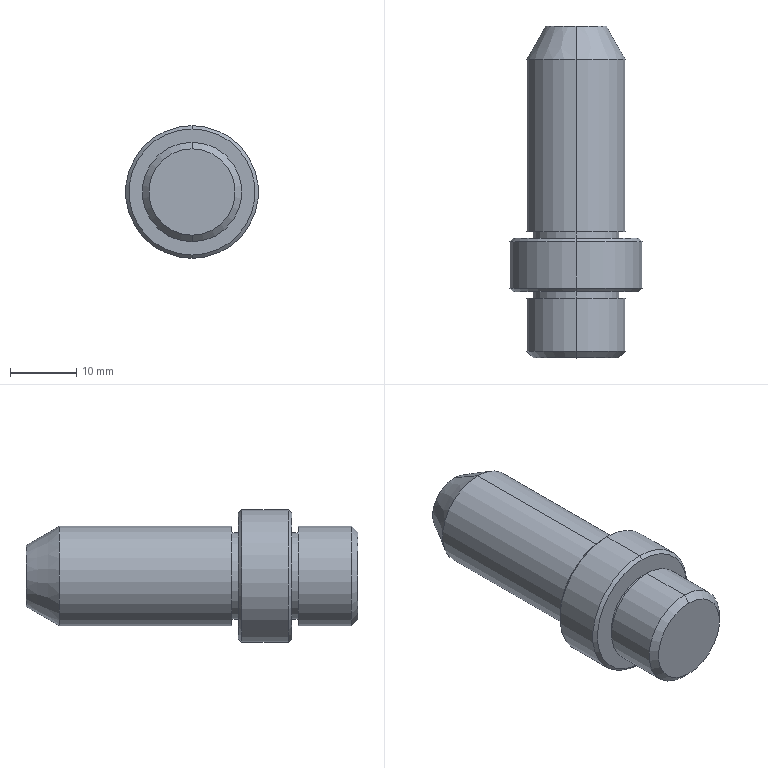Part | STEP file | Locating Pin | 1 solid | 24 faces | box 20 x 50 x 20 mm | volume 9513 mm3 | cylinder 10 | cone 8 | plane 6 | commonest cylinder face diameters 13 x4 15 x4 20 x2
STEP:
#1=CARTESIAN_POINT('',(0.,0.,0.));
#2=DIRECTION('',(0.,0.,1.));
#3=DIRECTION('',(1.,0.,0.));
#4=AXIS2_PLACEMENT_3D('',#1,#2,#3);
#5=CARTESIAN_POINT('',(18051.815,6151.815,9.5));
#6=VERTEX_POINT('',#5);
#7=CARTESIAN_POINT('',(18051.815,6151.815,-9.5));
#8=VERTEX_POINT('',#7);
#9=CARTESIAN_POINT('',(18051.815,6151.815,0.));
#10=DIRECTION('',(0.,1.,0.));
#11=DIRECTION('',(0.,0.,-1.));
#12=AXIS2_PLACEMENT_3D('',#9,#10,#11);
#13=CIRCLE('',#12,9.5);
#14=CARTESIAN_POINT('',(18051.815,6151.315,0.));
#15=DIRECTION('',(0.,-1.,0.));
#16=DIRECTION('',(0.,0.,-1.));
#17=AXIS2_PLACEMENT_3D('',#14,#15,#16);
#18=CONICAL_SURFACE('',#17,10.,0.7854);
#19=CARTESIAN_POINT('',(6.283,-0.5));
#20=DIRECTION('',(-1.,0.));
#21=VECTOR('',#20,1.);
#22=LINE('',#19,#21);
#23=(GEOMETRIC_REPRESENTATION_CONTEXT(2)PARAMETRIC_REPRESENTATION_CONTEXT()REPRESENTATION_CONTEXT('',''));
#24=DEFINITIONAL_REPRESENTATION('',(#22),#23);
#25=PCURVE('',#18,#24);
#26=CARTESIAN_POINT('',(18063.315,6151.815,0.));
#27=DIRECTION('',(0.,-1.,0.));
#28=DIRECTION('',(0.,0.,-1.));
#29=AXIS2_PLACEMENT_3D('',#26,#27,#28);
#30=PLANE('',#29);
#31=CARTESIAN_POINT('',(9.5,-11.5));
#32=CARTESIAN_POINT('',(9.5,-27.954));
#33=CARTESIAN_POINT('',(-4.75,-19.727));
#34=CARTESIAN_POINT('',(-19.,-11.5));
#35=CARTESIAN_POINT('',(-4.75,-3.273));
#36=CARTESIAN_POINT('',(9.5,4.954));
#37=CARTESIAN_POINT('',(9.5,-11.5));
#38=(BOUNDED_CURVE()B_SPLINE_CURVE(2,(#31,#32,#33,#34,#35,#36,#37),.UNSPECIFIED.,.T.,.F.)B_SPLINE_CURVE_WITH_KNOTS((1,2,2,2,2,1),(-2.094,0.,2.094,4.189,6.283,8.378),.UNSPECIFIED.)CURVE()GEOMETRIC_REPRESENTATION_ITEM()RATIONAL_B_SPLINE_CURVE((1.,0.5,1.,0.5,1.,0.5,1.))REPRESENTATION_ITEM(''));
#39=(GEOMETRIC_REPRESENTATION_CONTEXT(2)PARAMETRIC_REPRESENTATION_CONTEXT()REPRESENTATION_CONTEXT('',''));
#40=DEFINITIONAL_REPRESENTATION('',(#38),#39);
#41=PCURVE('',#30,#40);
#42=SURFACE_CURVE('',#13,(#25,#41),.PCURVE_S1.);
#43=EDGE_CURVE('',#6,#8,#42,.T.);
#44=ORIENTED_EDGE('',*,*,#43,.F.);
#45=CARTESIAN_POINT('',(18051.815,6151.315,10.));
#46=VERTEX_POINT('',#45);
#47=CARTESIAN_POINT('',(18051.815,6151.315,10.));
#48=DIRECTION('',(0.,-0.7071,0.7071));
#49=VECTOR('',#48,1.);
#50=LINE('',#47,#49);
#51=CARTESIAN_POINT('',(3.142,0.));
#52=DIRECTION('',(0.,1.));
#53=VECTOR('',#52,1.);
#54=LINE('',#51,#53);
#55=(GEOMETRIC_REPRESENTATION_CONTEXT(2)PARAMETRIC_REPRESENTATION_CONTEXT()REPRESENTATION_CONTEXT('',''));
#56=DEFINITIONAL_REPRESENTATION('',(#54),#55);
#57=PCURVE('',#18,#56);
#58=CARTESIAN_POINT('',(18051.815,6151.315,0.));
#59=DIRECTION('',(0.,-1.,0.));
#60=DIRECTION('',(0.,0.,-1.));
#61=AXIS2_PLACEMENT_3D('',#58,#59,#60);
#62=CONICAL_SURFACE('',#61,10.,0.7854);
#63=CARTESIAN_POINT('',(3.142,0.));
#64=DIRECTION('',(0.,1.));
#65=VECTOR('',#64,1.);
#66=LINE('',#63,#65);
#67=(GEOMETRIC_REPRESENTATION_CONTEXT(2)PARAMETRIC_REPRESENTATION_CONTEXT()REPRESENTATION_CONTEXT('',''));
#68=DEFINITIONAL_REPRESENTATION('',(#66),#67);
#69=PCURVE('',#62,#68);
#70=SURFACE_CURVE('',#50,(#57,#69),.PCURVE_S1.);
#71=EDGE_CURVE('',#6,#46,#70,.T.);
#72=ORIENTED_EDGE('',*,*,#71,.T.);
#73=CARTESIAN_POINT('',(18051.815,6151.315,-10.));
#74=VERTEX_POINT('',#73);
#75=CARTESIAN_POINT('',(18051.815,6151.315,0.));
#76=DIRECTION('',(0.,-1.,0.));
#77=DIRECTION('',(0.,0.,-1.));
#78=AXIS2_PLACEMENT_3D('',#75,#76,#77);
#79=CIRCLE('',#78,10.);
#80=CARTESIAN_POINT('',(0.,0.));
#81=DIRECTION('',(1.,0.));
#82=VECTOR('',#81,1.);
#83=LINE('',#80,#82);
#84=(GEOMETRIC_REPRESENTATION_CONTEXT(2)PARAMETRIC_REPRESENTATION_CONTEXT()REPRESENTATION_CONTEXT('',''));
#85=DEFINITIONAL_REPRESENTATION('',(#83),#84);
#86=PCURVE('',#18,#85);
#87=CARTESIAN_POINT('',(18051.815,6134.815,0.));
#88=DIRECTION('',(0.,1.,0.));
#89=DIRECTION('',(0.,0.,1.));
#90=AXIS2_PLACEMENT_3D('',#87,#88,#89);
#91=CYLINDRICAL_SURFACE('',#90,10.);
#92=CARTESIAN_POINT('',(3.142,16.5));
#93=DIRECTION('',(-1.,0.));
#94=VECTOR('',#93,1.);
#95=LINE('',#92,#94);
#96=(GEOMETRIC_REPRESENTATION_CONTEXT(2)PARAMETRIC_REPRESENTATION_CONTEXT()REPRESENTATION_CONTEXT('',''));
#97=DEFINITIONAL_REPRESENTATION('',(#95),#96);
#98=PCURVE('',#91,#97);
#99=SURFACE_CURVE('',#79,(#86,#98),.PCURVE_S1.);
#100=EDGE_CURVE('',#74,#46,#99,.T.);
#101=ORIENTED_EDGE('',*,*,#100,.F.);
#102=CARTESIAN_POINT('',(18051.815,6151.315,-10.));
#103=DIRECTION('',(0.,-0.7071,-0.7071));
#104=VECTOR('',#103,1.);
#105=LINE('',#102,#104);
#106=CARTESIAN_POINT('',(0.,0.));
#107=DIRECTION('',(0.,1.));
#108=VECTOR('',#107,1.);
#109=LINE('',#106,#108);
#110=(GEOMETRIC_REPRESENTATION_CONTEXT(2)PARAMETRIC_REPRESENTATION_CONTEXT()REPRESENTATION_CONTEXT('',''));
#111=DEFINITIONAL_REPRESENTATION('',(#109),#110);
#112=PCURVE('',#18,#111);
#113=CARTESIAN_POINT('',(6.283,0.));
#114=DIRECTION('',(0.,1.));
#115=VECTOR('',#114,1.);
#116=LINE('',#113,#115);
#117=(GEOMETRIC_REPRESENTATION_CONTEXT(2)PARAMETRIC_REPRESENTATION_CONTEXT()REPRESENTATION_CONTEXT('',''));
#118=DEFINITIONAL_REPRESENTATION('',(#116),#117);
#119=PCURVE('',#62,#118);
#120=SURFACE_CURVE('',#105,(#112,#119),.PCURVE_S1.);
#121=EDGE_CURVE('',#8,#74,#120,.T.);
#122=ORIENTED_EDGE('',*,*,#121,.F.);
#123=EDGE_LOOP('',(#44,#72,#101,#122));
#124=FACE_BOUND('',#123,.T.);
#125=ADVANCED_FACE('',(#124),#18,.T.);
#126=CARTESIAN_POINT('',(18051.815,6143.815,-9.5));
#127=VERTEX_POINT('',#126);
#128=CARTESIAN_POINT('',(18051.815,6143.815,9.5));
#129=VERTEX_POINT('',#128);
#130=CARTESIAN_POINT('',(18051.815,6143.815,0.));
#131=DIRECTION('',(0.,-1.,0.));
#132=DIRECTION('',(0.,0.,1.));
#133=AXIS2_PLACEMENT_3D('',#130,#131,#132);
#134=CIRCLE('',#133,9.5);
#135=CARTESIAN_POINT('',(18051.815,6144.315,0.));
#136=DIRECTION('',(0.,1.,0.));
#137=DIRECTION('',(0.,0.,1.));
#138=AXIS2_PLACEMENT_3D('',#135,#136,#137);
#139=CONICAL_SURFACE('',#138,10.,0.7854);
#140=CARTESIAN_POINT('',(6.283,-0.5));
#141=DIRECTION('',(-1.,0.));
#142=VECTOR('',#141,1.);
#143=LINE('',#140,#142);
#144=(GEOMETRIC_REPRESENTATION_CONTEXT(2)PARAMETRIC_REPRESENTATION_CONTEXT()REPRESENTATION_CONTEXT('',''));
#145=DEFINITIONAL_REPRESENTATION('',(#143),#144);
#146=PCURVE('',#139,#145);
#147=CARTESIAN_POINT('',(18058.315,6143.815,0.));
#148=DIRECTION('',(0.,1.,0.));
#149=DIRECTION('',(0.,0.,1.));
#150=AXIS2_PLACEMENT_3D('',#147,#148,#149);
#151=PLANE('',#150);
#152=CARTESIAN_POINT('',(9.5,-6.5));
#153=CARTESIAN_POINT('',(9.5,-22.954));
#154=CARTESIAN_POINT('',(-4.75,-14.727));
#155=CARTESIAN_POINT('',(-19.,-6.5));
#156=CARTESIAN_POINT('',(-4.75,1.727));
#157=CARTESIAN_POINT('',(9.5,9.954));
#158=CARTESIAN_POINT('',(9.5,-6.5));
#159=(BOUNDED_CURVE()B_SPLINE_CURVE(2,(#152,#153,#154,#155,#156,#157,#158),.UNSPECIFIED.,.T.,.F.)B_SPLINE_CURVE_WITH_KNOTS((1,2,2,2,2,1),(-2.094,0.,2.094,4.189,6.283,8.378),.UNSPECIFIED.)CURVE()GEOMETRIC_REPRESENTATION_ITEM()RATIONAL_B_SPLINE_CURVE((1.,0.5,1.,0.5,1.,0.5,1.))REPRESENTATION_ITEM(''));
#160=(GEOMETRIC_REPRESENTATION_CONTEXT(2)PARAMETRIC_REPRESENTATION_CONTEXT()REPRESENTATION_CONTEXT('',''));
#161=DEFINITIONAL_REPRESENTATION('',(#159),#160);
#162=PCURVE('',#151,#161);
#163=SURFACE_CURVE('',#134,(#146,#162),.PCURVE_S1.);
#164=EDGE_CURVE('',#127,#129,#163,.T.);
#165=ORIENTED_EDGE('',*,*,#164,.F.);
#166=CARTESIAN_POINT('',(18051.815,6144.315,-10.));
#167=VERTEX_POINT('',#166);
#168=CARTESIAN_POINT('',(18051.815,6144.315,-10.));
#169=DIRECTION('',(0.,0.7071,-0.7071));
#170=VECTOR('',#169,1.);
#171=LINE('',#168,#170);
#172=CARTESIAN_POINT('',(3.142,0.));
#173=DIRECTION('',(0.,1.));
#174=VECTOR('',#173,1.);
#175=LINE('',#172,#174);
#176=(GEOMETRIC_REPRESENTATION_CONTEXT(2)PARAMETRIC_REPRESENTATION_CONTEXT()REPRESENTATION_CONTEXT('',''));
#177=DEFINITIONAL_REPRESENTATION('',(#175),#176);
#178=PCURVE('',#139,#177);
#179=CARTESIAN_POINT('',(18051.815,6144.315,0.));
#180=DIRECTION('',(0.,1.,0.));
#181=DIRECTION('',(0.,0.,1.));
#182=AXIS2_PLACEMENT_3D('',#179,#180,#181);
#183=CONICAL_SURFACE('',#182,10.,0.7854);
#184=CARTESIAN_POINT('',(3.142,0.));
#185=DIRECTION('',(0.,1.));
#186=VECTOR('',#185,1.);
#187=LINE('',#184,#186);
#188=(GEOMETRIC_REPRESENTATION_CONTEXT(2)PARAMETRIC_REPRESENTATION_CONTEXT()REPRESENTATION_CONTEXT('',''));
#189=DEFINITIONAL_REPRESENTATION('',(#187),#188);
#190=PCURVE('',#183,#189);
#191=SURFACE_CURVE('',#171,(#178,#190),.PCURVE_S1.);
#192=EDGE_CURVE('',#127,#167,#191,.T.);
#193=ORIENTED_EDGE('',*,*,#192,.T.);
#194=CARTESIAN_POINT('',(18051.815,6144.315,10.));
#195=VERTEX_POINT('',#194);
#196=CARTESIAN_POINT('',(18051.815,6144.315,0.));
#197=DIRECTION('',(0.,1.,0.));
#198=DIRECTION('',(0.,0.,1.));
#199=AXIS2_PLACEMENT_3D('',#196,#197,#198);
#200=CIRCLE('',#199,10.);
#201=CARTESIAN_POINT('',(0.,0.));
#202=DIRECTION('',(1.,0.));
#203=VECTOR('',#202,1.);
#204=LINE('',#201,#203);
#205=(GEOMETRIC_REPRESENTATION_CONTEXT(2)PARAMETRIC_REPRESENTATION_CONTEXT()REPRESENTATION_CONTEXT('',''));
#206=DEFINITIONAL_REPRESENTATION('',(#204),#205);
#207=PCURVE('',#139,#206);
#208=CARTESIAN_POINT('',(0.,9.5));
#209=DIRECTION('',(1.,0.));
#210=VECTOR('',#209,1.);
#211=LINE('',#208,#210);
#212=(GEOMETRIC_REPRESENTATION_CONTEXT(2)PARAMETRIC_REPRESENTATION_CONTEXT()REPRESENTATION_CONTEXT('',''));
#213=DEFINITIONAL_REPRESENTATION('',(#211),#212);
#214=PCURVE('',#91,#213);
#215=SURFACE_CURVE('',#200,(#207,#214),.PCURVE_S1.);
#216=EDGE_CURVE('',#195,#167,#215,.T.);
#217=ORIENTED_EDGE('',*,*,#216,.F.);
#218=CARTESIAN_POINT('',(18051.815,6144.315,10.));
#219=DIRECTION('',(0.,0.7071,0.7071));
#220=VECTOR('',#219,1.);
#221=LINE('',#218,#220);
#222=CARTESIAN_POINT('',(0.,0.));
#223=DIRECTION('',(0.,1.));
#224=VECTOR('',#223,1.);
#225=LINE('',#222,#224);
#226=(GEOMETRIC_REPRESENTATION_CONTEXT(2)PARAMETRIC_REPRESENTATION_CONTEXT()REPRESENTATION_CONTEXT('',''));
#227=DEFINITIONAL_REPRESENTATION('',(#225),#226);
#228=PCURVE('',#139,#227);
#229=CARTESIAN_POINT('',(6.283,0.));
#230=DIRECTION('',(0.,1.));
#231=VECTOR('',#230,1.);
#232=LINE('',#229,#231);
#233=(GEOMETRIC_REPRESENTATION_CONTEXT(2)PARAMETRIC_REPRESENTATION_CONTEXT()REPRESENTATION_CONTEXT('',''));
#234=DEFINITIONAL_REPRESENTATION('',(#232),#233);
#235=PCURVE('',#183,#234);
#236=SURFACE_CURVE('',#221,(#228,#235),.PCURVE_S1.);
#237=EDGE_CURVE('',#129,#195,#236,.T.);
#238=ORIENTED_EDGE('',*,*,#237,.F.);
#239=EDGE_LOOP('',(#165,#193,#217,#238));
#240=FACE_BOUND('',#239,.T.);
#241=ADVANCED_FACE('',(#240),#139,.T.);
#242=CARTESIAN_POINT('',(18051.815,6142.815,6.5));
#243=VERTEX_POINT('',#242);
#244=CARTESIAN_POINT('',(18051.815,6142.815,-6.5));
#245=VERTEX_POINT('',#244);
#246=CARTESIAN_POINT('',(18051.815,6142.815,0.));
#247=DIRECTION('',(0.,1.,0.));
#248=DIRECTION('',(0.,0.,1.));
#249=AXIS2_PLACEMENT_3D('',#246,#247,#248);
#250=CIRCLE('',#249,6.5);
#251=CARTESIAN_POINT('',(18051.815,6187.914,0.));
#252=DIRECTION('',(0.,1.,0.));
#253=DIRECTION('',(0.,0.,1.));
#254=AXIS2_PLACEMENT_3D('',#251,#252,#253);
#255=CYLINDRICAL_SURFACE('',#254,6.5);
#256=CARTESIAN_POINT('',(0.,-45.099));
#257=DIRECTION('',(1.,0.));
#258=VECTOR('',#257,1.);
#259=LINE('',#256,#258);
#260=(GEOMETRIC_REPRESENTATION_CONTEXT(2)PARAMETRIC_REPRESENTATION_CONTEXT()REPRESENTATION_CONTEXT('',''));
#261=DEFINITIONAL_REPRESENTATION('',(#259),#260);
#262=PCURVE('',#255,#261);
#263=CARTESIAN_POINT('',(18059.315,6142.815,0.));
#264=DIRECTION('',(0.,-1.,0.));
#265=DIRECTION('',(0.,0.,-1.));
#266=AXIS2_PLACEMENT_3D('',#263,#264,#265);
#267=PLANE('',#266);
#268=CARTESIAN_POINT('',(-6.5,-7.5));
#269=CARTESIAN_POINT('',(-6.5,3.758));
#270=CARTESIAN_POINT('',(3.25,-1.871));
#271=CARTESIAN_POINT('',(13.,-7.5));
#272=CARTESIAN_POINT('',(3.25,-13.129));
#273=CARTESIAN_POINT('',(-6.5,-18.758));
#274=CARTESIAN_POINT('',(-6.5,-7.5));
#275=(BOUNDED_CURVE()B_SPLINE_CURVE(2,(#268,#269,#270,#271,#272,#273,#274),.UNSPECIFIED.,.T.,.F.)B_SPLINE_CURVE_WITH_KNOTS((1,2,2,2,2,1),(-2.094,0.,2.094,4.189,6.283,8.378),.UNSPECIFIED.)CURVE()GEOMETRIC_REPRESENTATION_ITEM()RATIONAL_B_SPLINE_CURVE((1.,0.5,1.,0.5,1.,0.5,1.))REPRESENTATION_ITEM(''));
#276=(GEOMETRIC_REPRESENTATION_CONTEXT(2)PARAMETRIC_REPRESENTATION_CONTEXT()REPRESENTATION_CONTEXT('',''));
#277=DEFINITIONAL_REPRESENTATION('',(#275),#276);
#278=PCURVE('',#267,#277);
#279=SURFACE_CURVE('',#250,(#262,#278),.PCURVE_S1.);
#280=EDGE_CURVE('',#243,#245,#279,.T.);
#281=ORIENTED_EDGE('',*,*,#280,.T.);
#282=CARTESIAN_POINT('',(18051.815,6143.815,-6.5));
#283=VERTEX_POINT('',#282);
#284=CARTESIAN_POINT('',(18051.815,6187.914,-6.5));
#285=DIRECTION('',(0.,1.,0.));
#286=VECTOR('',#285,1.);
#287=LINE('',#284,#286);
#288=CARTESIAN_POINT('',(3.142,0.));
#289=DIRECTION('',(0.,1.));
#290=VECTOR('',#289,1.);
#291=LINE('',#288,#290);
#292=(GEOMETRIC_REPRESENTATION_CONTEXT(2)PARAMETRIC_REPRESENTATION_CONTEXT()REPRESENTATION_CONTEXT('',''));
#293=DEFINITIONAL_REPRESENTATION('',(#291),#292);
#294=PCURVE('',#255,#293);
#295=CARTESIAN_POINT('',(18051.815,6187.914,0.));
#296=DIRECTION('',(0.,1.,0.));
#297=DIRECTION('',(0.,0.,1.));
#298=AXIS2_PLACEMENT_3D('',#295,#296,#297);
#299=CYLINDRICAL_SURFACE('',#298,6.5);
#300=CARTESIAN_POINT('',(3.142,0.));
#301=DIRECTION('',(0.,1.));
#302=VECTOR('',#301,1.);
#303=LINE('',#300,#302);
#304=(GEOMETRIC_REPRESENTATION_CONTEXT(2)PARAMETRIC_REPRESENTATION_CONTEXT()REPRESENTATION_CONTEXT('',''));
#305=DEFINITIONAL_REPRESENTATION('',(#303),#304);
#306=PCURVE('',#299,#305);
#307=SURFACE_CURVE('',#287,(#294,#306),.PCURVE_S1.);
#308=EDGE_CURVE('',#245,#283,#307,.T.);
#309=ORIENTED_EDGE('',*,*,#308,.T.);
#310=CARTESIAN_POINT('',(18051.815,6143.815,6.5));
#311=VERTEX_POINT('',#310);
#312=CARTESIAN_POINT('',(18051.815,6143.815,0.));
#313=DIRECTION('',(0.,1.,0.));
#314=DIRECTION('',(0.,0.,1.));
#315=AXIS2_PLACEMENT_3D('',#312,#313,#314);
#316=CIRCLE('',#315,6.5);
#317=CARTESIAN_POINT('',(0.,-44.099));
#318=DIRECTION('',(1.,0.));
#319=VECTOR('',#318,1.);
#320=LINE('',#317,#319);
#321=(GEOMETRIC_REPRESENTATION_CONTEXT(2)PARAMETRIC_REPRESENTATION_CONTEXT()REPRESENTATION_CONTEXT('',''));
#322=DEFINITIONAL_REPRESENTATION('',(#320),#321);
#323=PCURVE('',#255,#322);
#324=CARTESIAN_POINT('',(0.,-6.5));
#325=DIRECTION('',(1.,0.));
#326=AXIS2_PLACEMENT_2D('',#324,#325);
#327=CIRCLE('',#326,6.5);
#328=(GEOMETRIC_REPRESENTATION_CONTEXT(2)PARAMETRIC_REPRESENTATION_CONTEXT()REPRESENTATION_CONTEXT('',''));
#329=DEFINITIONAL_REPRESENTATION('',(#327),#328);
#330=PCURVE('',#151,#329);
#331=SURFACE_CURVE('',#316,(#323,#330),.PCURVE_S1.);
#332=EDGE_CURVE('',#311,#283,#331,.T.);
#333=ORIENTED_EDGE('',*,*,#332,.F.);
#334=CARTESIAN_POINT('',(18051.815,6187.914,6.5));
#335=DIRECTION('',(0.,1.,0.));
#336=VECTOR('',#335,1.);
#337=LINE('',#334,#336);
#338=CARTESIAN_POINT('',(0.,0.));
#339=DIRECTION('',(0.,1.));
#340=VECTOR('',#339,1.);
#341=LINE('',#338,#340);
#342=(GEOMETRIC_REPRESENTATION_CONTEXT(2)PARAMETRIC_REPRESENTATION_CONTEXT()REPRESENTATION_CONTEXT('',''));
#343=DEFINITIONAL_REPRESENTATION('',(#341),#342);
#344=PCURVE('',#255,#343);
#345=CARTESIAN_POINT('',(6.283,0.));
#346=DIRECTION('',(0.,1.));
#347=VECTOR('',#346,1.);
#348=LINE('',#345,#347);
#349=(GEOMETRIC_REPRESENTATION_CONTEXT(2)PARAMETRIC_REPRESENTATION_CONTEXT()REPRESENTATION_CONTEXT('',''));
#350=DEFINITIONAL_REPRESENTATION('',(#348),#349);
#351=PCURVE('',#299,#350);
#352=SURFACE_CURVE('',#337,(#344,#351),.PCURVE_S1.);
#353=EDGE_CURVE('',#243,#311,#352,.T.);
#354=ORIENTED_EDGE('',*,*,#353,.F.);
#355=EDGE_LOOP('',(#281,#309,#333,#354));
#356=FACE_BOUND('',#355,.T.);
#357=ADVANCED_FACE('',(#356),#255,.T.);
#358=CARTESIAN_POINT('',(18051.815,6134.815,7.5));
#359=VERTEX_POINT('',#358);
#360=CARTESIAN_POINT('',(18051.815,6134.815,-7.5));
#361=VERTEX_POINT('',#360);
#362=CARTESIAN_POINT('',(18051.815,6134.815,0.));
#363=DIRECTION('',(0.,1.,0.));
#364=DIRECTION('',(0.,0.,1.));
#365=AXIS2_PLACEMENT_3D('',#362,#363,#364);
#366=CIRCLE('',#365,7.5);
#367=CARTESIAN_POINT('',(18051.815,6187.914,0.));
#368=DIRECTION('',(0.,1.,0.));
#369=DIRECTION('',(0.,0.,1.));
#370=AXIS2_PLACEMENT_3D('',#367,#368,#369);
#371=CYLINDRICAL_SURFACE('',#370,7.5);
#372=CARTESIAN_POINT('',(0.,-53.099));
#373=DIRECTION('',(1.,0.));
#374=VECTOR('',#373,1.);
#375=LINE('',#372,#374);
#376=(GEOMETRIC_REPRESENTATION_CONTEXT(2)PARAMETRIC_REPRESENTATION_CONTEXT()REPRESENTATION_CONTEXT('',''));
#377=DEFINITIONAL_REPRESENTATION('',(#375),#376);
#378=PCURVE('',#371,#377);
#379=CARTESIAN_POINT('',(18051.815,6133.815,0.));
#380=DIRECTION('',(0.,1.,0.));
#381=DIRECTION('',(0.,0.,1.));
#382=AXIS2_PLACEMENT_3D('',#379,#380,#381);
#383=CONICAL_SURFACE('',#382,6.5,0.7854);
#384=CARTESIAN_POINT('',(0.,1.));
#385=DIRECTION('',(1.,0.));
#386=VECTOR('',#385,1.);
#387=LINE('',#384,#386);
#388=(GEOMETRIC_REPRESENTATION_CONTEXT(2)PARAMETRIC_REPRESENTATION_CONTEXT()REPRESENTATION_CONTEXT('',''));
#389=DEFINITIONAL_REPRESENTATION('',(#387),#388);
#390=PCURVE('',#383,#389);
#391=SURFACE_CURVE('',#366,(#378,#390),.PCURVE_S1.);
#392=EDGE_CURVE('',#359,#361,#391,.T.);
#393=ORIENTED_EDGE('',*,*,#392,.T.);
#394=CARTESIAN_POINT('',(18051.815,6142.815,-7.5));
#395=VERTEX_POINT('',#394);
#396=CARTESIAN_POINT('',(18051.815,6187.914,-7.5));
#397=DIRECTION('',(0.,1.,0.));
#398=VECTOR('',#397,1.);
#399=LINE('',#396,#398);
#400=CARTESIAN_POINT('',(3.142,0.));
#401=DIRECTION('',(0.,1.));
#402=VECTOR('',#401,1.);
#403=LINE('',#400,#402);
#404=(GEOMETRIC_REPRESENTATION_CONTEXT(2)PARAMETRIC_REPRESENTATION_CONTEXT()REPRESENTATION_CONTEXT('',''));
#405=DEFINITIONAL_REPRESENTATION('',(#403),#404);
#406=PCURVE('',#371,#405);
#407=CARTESIAN_POINT('',(18051.815,6187.914,0.));
#408=DIRECTION('',(0.,1.,0.));
#409=DIRECTION('',(0.,0.,1.));
#410=AXIS2_PLACEMENT_3D('',#407,#408,#409);
#411=CYLINDRICAL_SURFACE('',#410,7.5);
#412=CARTESIAN_POINT('',(3.142,0.));
#413=DIRECTION('',(0.,1.));
#414=VECTOR('',#413,1.);
#415=LINE('',#412,#414);
#416=(GEOMETRIC_REPRESENTATION_CONTEXT(2)PARAMETRIC_REPRESENTATION_CONTEXT()REPRESENTATION_CONTEXT('',''));
#417=DEFINITIONAL_REPRESENTATION('',(#415),#416);
#418=PCURVE('',#411,#417);
#419=SURFACE_CURVE('',#399,(#406,#418),.PCURVE_S1.);
#420=EDGE_CURVE('',#361,#395,#419,.T.);
#421=ORIENTED_EDGE('',*,*,#420,.T.);
#422=CARTESIAN_POINT('',(18051.815,6142.815,7.5));
#423=VERTEX_POINT('',#422);
#424=CARTESIAN_POINT('',(18051.815,6142.815,0.));
#425=DIRECTION('',(0.,1.,0.));
#426=DIRECTION('',(0.,0.,1.));
#427=AXIS2_PLACEMENT_3D('',#424,#425,#426);
#428=CIRCLE('',#427,7.5);
#429=CARTESIAN_POINT('',(0.,-45.099));
#430=DIRECTION('',(1.,0.));
#431=VECTOR('',#430,1.);
#432=LINE('',#429,#431);
#433=(GEOMETRIC_REPRESENTATION_CONTEXT(2)PARAMETRIC_REPRESENTATION_CONTEXT()REPRESENTATION_CONTEXT('',''));
#434=DEFINITIONAL_REPRESENTATION('',(#432),#433);
#435=PCURVE('',#371,#434);
#436=CARTESIAN_POINT('',(-7.5,-7.5));
#437=CARTESIAN_POINT('',(-7.5,5.49));
#438=CARTESIAN_POINT('',(3.75,-1.005));
#439=CARTESIAN_POINT('',(15.,-7.5));
#440=CARTESIAN_POINT('',(3.75,-13.995));
#441=CARTESIAN_POINT('',(-7.5,-20.49));
#442=CARTESIAN_POINT('',(-7.5,-7.5));
#443=(BOUNDED_CURVE()B_SPLINE_CURVE(2,(#436,#437,#438,#439,#440,#441,#442),.UNSPECIFIED.,.T.,.F.)B_SPLINE_CURVE_WITH_KNOTS((1,2,2,2,2,1),(-2.094,0.,2.094,4.189,6.283,8.378),.UNSPECIFIED.)CURVE()GEOMETRIC_REPRESENTATION_ITEM()RATIONAL_B_SPLINE_CURVE((1.,0.5,1.,0.5,1.,0.5,1.))REPRESENTATION_ITEM(''));
#444=(GEOMETRIC_REPRESENTATION_CONTEXT(2)PARAMETRIC_REPRESENTATION_CONTEXT()REPRESENTATION_CONTEXT('',''));
#445=DEFINITIONAL_REPRESENTATION('',(#443),#444);
#446=PCURVE('',#267,#445);
#447=SURFACE_CURVE('',#428,(#435,#446),.PCURVE_S1.);
#448=EDGE_CURVE('',#423,#395,#447,.T.);
#449=ORIENTED_EDGE('',*,*,#448,.F.);
#450=CARTESIAN_POINT('',(18051.815,6187.914,7.5));
#451=DIRECTION('',(0.,1.,0.));
#452=VECTOR('',#451,1.);
#453=LINE('',#450,#452);
#454=CARTESIAN_POINT('',(0.,0.));
#455=DIRECTION('',(0.,1.));
#456=VECTOR('',#455,1.);
#457=LINE('',#454,#456);
#458=(GEOMETRIC_REPRESENTATION_CONTEXT(2)PARAMETRIC_REPRESENTATION_CONTEXT()REPRESENTATION_CONTEXT('',''));
#459=DEFINITIONAL_REPRESENTATION('',(#457),#458);
#460=PCURVE('',#371,#459);
#461=CARTESIAN_POINT('',(6.283,0.));
#462=DIRECTION('',(0.,1.));
#463=VECTOR('',#462,1.);
#464=LINE('',#461,#463);
#465=(GEOMETRIC_REPRESENTATION_CONTEXT(2)PARAMETRIC_REPRESENTATION_CONTEXT()REPRESENTATION_CONTEXT('',''));
#466=DEFINITIONAL_REPRESENTATION('',(#464),#465);
#467=PCURVE('',#411,#466);
#468=SURFACE_CURVE('',#453,(#460,#467),.PCURVE_S1.);
#469=EDGE_CURVE('',#359,#423,#468,.T.);
#470=ORIENTED_EDGE('',*,*,#469,.F.);
#471=EDGE_LOOP('',(#393,#421,#449,#470));
#472=FACE_BOUND('',#471,.T.);
#473=ADVANCED_FACE('',(#472),#371,.T.);
#474=CARTESIAN_POINT('',(18051.815,6133.815,6.5));
#475=VERTEX_POINT('',#474);
#476=CARTESIAN_POINT('',(18051.815,6133.815,-6.5));
#477=VERTEX_POINT('',#476);
#478=CARTESIAN_POINT('',(18051.815,6133.815,0.));
#479=DIRECTION('',(0.,1.,0.));
#480=DIRECTION('',(0.,0.,1.));
#481=AXIS2_PLACEMENT_3D('',#478,#479,#480);
#482=CIRCLE('',#481,6.5);
#483=CARTESIAN_POINT('',(0.,0.));
#484=DIRECTION('',(1.,0.));
#485=VECTOR('',#484,1.);
#486=LINE('',#483,#485);
#487=(GEOMETRIC_REPRESENTATION_CONTEXT(2)PARAMETRIC_REPRESENTATION_CONTEXT()REPRESENTATION_CONTEXT('',''));
#488=DEFINITIONAL_REPRESENTATION('',(#486),#487);
#489=PCURVE('',#383,#488);
#490=CARTESIAN_POINT('',(18058.315,6133.815,0.));
#491=DIRECTION('',(0.,1.,0.));
#492=DIRECTION('',(0.,0.,1.));
#493=AXIS2_PLACEMENT_3D('',#490,#491,#492);
#494=PLANE('',#493);
#495=CARTESIAN_POINT('',(0.,-6.5));
#496=DIRECTION('',(1.,0.));
#497=AXIS2_PLACEMENT_2D('',#495,#496);
#498=CIRCLE('',#497,6.5);
#499=(GEOMETRIC_REPRESENTATION_CONTEXT(2)PARAMETRIC_REPRESENTATION_CONTEXT()REPRESENTATION_CONTEXT('',''));
#500=DEFINITIONAL_REPRESENTATION('',(#498),#499);
#501=PCURVE('',#494,#500);
#502=SURFACE_CURVE('',#482,(#489,#501),.PCURVE_S1.);
#503=EDGE_CURVE('',#475,#477,#502,.T.);
#504=ORIENTED_EDGE('',*,*,#503,.T.);
#505=CARTESIAN_POINT('',(18051.815,6133.815,-6.5));
#506=DIRECTION('',(0.,0.7071,-0.7071));
#507=VECTOR('',#506,1.);
#508=LINE('',#505,#507);
#509=CARTESIAN_POINT('',(3.142,0.));
#510=DIRECTION('',(0.,1.));
#511=VECTOR('',#510,1.);
#512=LINE('',#509,#511);
#513=(GEOMETRIC_REPRESENTATION_CONTEXT(2)PARAMETRIC_REPRESENTATION_CONTEXT()REPRESENTATION_CONTEXT('',''));
#514=DEFINITIONAL_REPRESENTATION('',(#512),#513);
#515=PCURVE('',#383,#514);
#516=CARTESIAN_POINT('',(18051.815,6133.815,0.));
#517=DIRECTION('',(0.,1.,0.));
#518=DIRECTION('',(0.,0.,1.));
#519=AXIS2_PLACEMENT_3D('',#516,#517,#518);
#520=CONICAL_SURFACE('',#519,6.5,0.7854);
#521=CARTESIAN_POINT('',(3.142,0.));
#522=DIRECTION('',(0.,1.));
#523=VECTOR('',#522,1.);
#524=LINE('',#521,#523);
#525=(GEOMETRIC_REPRESENTATION_CONTEXT(2)PARAMETRIC_REPRESENTATION_CONTEXT()REPRESENTATION_CONTEXT('',''));
#526=DEFINITIONAL_REPRESENTATION('',(#524),#525);
#527=PCURVE('',#520,#526);
#528=SURFACE_CURVE('',#508,(#515,#527),.PCURVE_S1.);
#529=EDGE_CURVE('',#477,#361,#528,.T.);
#530=ORIENTED_EDGE('',*,*,#529,.T.);
#531=ORIENTED_EDGE('',*,*,#392,.F.);
#532=CARTESIAN_POINT('',(18051.815,6133.815,6.5));
#533=DIRECTION('',(0.,0.7071,0.7071));
#534=VECTOR('',#533,1.);
#535=LINE('',#532,#534);
#536=CARTESIAN_POINT('',(0.,0.));
#537=DIRECTION('',(0.,1.));
#538=VECTOR('',#537,1.);
#539=LINE('',#536,#538);
#540=(GEOMETRIC_REPRESENTATION_CONTEXT(2)PARAMETRIC_REPRESENTATION_CONTEXT()REPRESENTATION_CONTEXT('',''));
#541=DEFINITIONAL_REPRESENTATION('',(#539),#540);
#542=PCURVE('',#383,#541);
#543=CARTESIAN_POINT('',(6.283,0.));
#544=DIRECTION('',(0.,1.));
#545=VECTOR('',#544,1.);
#546=LINE('',#543,#545);
#547=(GEOMETRIC_REPRESENTATION_CONTEXT(2)PARAMETRIC_REPRESENTATION_CONTEXT()REPRESENTATION_CONTEXT('',''));
#548=DEFINITIONAL_REPRESENTATION('',(#546),#547);
#549=PCURVE('',#520,#548);
#550=SURFACE_CURVE('',#535,(#542,#549),.PCURVE_S1.);
#551=EDGE_CURVE('',#475,#359,#550,.T.);
#552=ORIENTED_EDGE('',*,*,#551,.F.);
#553=EDGE_LOOP('',(#504,#530,#531,#552));
#554=FACE_BOUND('',#553,.T.);
#555=ADVANCED_FACE('',(#554),#383,.T.);
#556=ORIENTED_EDGE('',*,*,#216,.T.);
#557=CARTESIAN_POINT('',(18051.815,6134.815,-10.));
#558=DIRECTION('',(0.,1.,0.));
#559=VECTOR('',#558,1.);
#560=LINE('',#557,#559);
#561=CARTESIAN_POINT('',(3.142,0.));
#562=DIRECTION('',(0.,1.));
#563=VECTOR('',#562,1.);
#564=LINE('',#561,#563);
#565=(GEOMETRIC_REPRESENTATION_CONTEXT(2)PARAMETRIC_REPRESENTATION_CONTEXT()REPRESENTATION_CONTEXT('',''));
#566=DEFINITIONAL_REPRESENTATION('',(#564),#565);
#567=PCURVE('',#91,#566);
#568=CARTESIAN_POINT('',(18051.815,6134.815,0.));
#569=DIRECTION('',(0.,1.,0.));
#570=DIRECTION('',(0.,0.,1.));
#571=AXIS2_PLACEMENT_3D('',#568,#569,#570);
#572=CYLINDRICAL_SURFACE('',#571,10.);
#573=CARTESIAN_POINT('',(3.142,0.));
#574=DIRECTION('',(0.,1.));
#575=VECTOR('',#574,1.);
#576=LINE('',#573,#575);
#577=(GEOMETRIC_REPRESENTATION_CONTEXT(2)PARAMETRIC_REPRESENTATION_CONTEXT()REPRESENTATION_CONTEXT('',''));
#578=DEFINITIONAL_REPRESENTATION('',(#576),#577);
#579=PCURVE('',#572,#578);
#580=SURFACE_CURVE('',#560,(#567,#579),.PCURVE_S1.);
#581=EDGE_CURVE('',#167,#74,#580,.T.);
#582=ORIENTED_EDGE('',*,*,#581,.T.);
#583=ORIENTED_EDGE('',*,*,#100,.T.);
#584=CARTESIAN_POINT('',(18051.815,6134.815,10.));
#585=DIRECTION('',(0.,1.,0.));
#586=VECTOR('',#585,1.);
#587=LINE('',#584,#586);
#588=CARTESIAN_POINT('',(0.,0.));
#589=DIRECTION('',(0.,1.));
#590=VECTOR('',#589,1.);
#591=LINE('',#588,#590);
#592=(GEOMETRIC_REPRESENTATION_CONTEXT(2)PARAMETRIC_REPRESENTATION_CONTEXT()REPRESENTATION_CONTEXT('',''));
#593=DEFINITIONAL_REPRESENTATION('',(#591),#592);
#594=PCURVE('',#91,#593);
#595=CARTESIAN_POINT('',(6.283,0.));
#596=DIRECTION('',(0.,1.));
#597=VECTOR('',#596,1.);
#598=LINE('',#595,#597);
#599=(GEOMETRIC_REPRESENTATION_CONTEXT(2)PARAMETRIC_REPRESENTATION_CONTEXT()REPRESENTATION_CONTEXT('',''));
#600=DEFINITIONAL_REPRESENTATION('',(#598),#599);
#601=PCURVE('',#572,#600);
#602=SURFACE_CURVE('',#587,(#594,#601),.PCURVE_S1.);
#603=EDGE_CURVE('',#195,#46,#602,.T.);
#604=ORIENTED_EDGE('',*,*,#603,.F.);
#605=EDGE_LOOP('',(#556,#582,#583,#604));
#606=FACE_BOUND('',#605,.T.);
#607=ADVANCED_FACE('',(#606),#91,.T.);
#608=CARTESIAN_POINT('',(18051.815,6183.815,4.613));
#609=VERTEX_POINT('',#608);
#610=CARTESIAN_POINT('',(18051.815,6183.815,-4.613));
#611=VERTEX_POINT('',#610);
#612=CARTESIAN_POINT('',(18051.815,6183.815,0.));
#613=DIRECTION('',(0.,1.,0.));
#614=DIRECTION('',(0.,0.,1.));
#615=AXIS2_PLACEMENT_3D('',#612,#613,#614);
#616=CIRCLE('',#615,4.613);
#617=CARTESIAN_POINT('',(18051.815,6178.815,0.));
#618=DIRECTION('',(0.,-1.,0.));
#619=DIRECTION('',(0.,0.,-1.));
#620=AXIS2_PLACEMENT_3D('',#617,#618,#619);
#621=CONICAL_SURFACE('',#620,7.5,0.5236);
#622=CARTESIAN_POINT('',(3.142,-5.));
#623=DIRECTION('',(-1.,0.));
#624=VECTOR('',#623,1.);
#625=LINE('',#622,#624);
#626=(GEOMETRIC_REPRESENTATION_CONTEXT(2)PARAMETRIC_REPRESENTATION_CONTEXT()REPRESENTATION_CONTEXT('',''));
#627=DEFINITIONAL_REPRESENTATION('',(#625),#626);
#628=PCURVE('',#621,#627);
#629=CARTESIAN_POINT('',(18056.428,6183.815,0.));
#630=DIRECTION('',(0.,-1.,0.));
#631=DIRECTION('',(0.,0.,-1.));
#632=AXIS2_PLACEMENT_3D('',#629,#630,#631);
#633=PLANE('',#632);
#634=CARTESIAN_POINT('',(-4.613,-4.613));
#635=CARTESIAN_POINT('',(-4.613,3.377));
#636=CARTESIAN_POINT('',(2.307,-0.6181));
#637=CARTESIAN_POINT('',(9.226,-4.613));
#638=CARTESIAN_POINT('',(2.307,-8.608));
#639=CARTESIAN_POINT('',(-4.613,-12.604));
#640=CARTESIAN_POINT('',(-4.613,-4.613));
#641=(BOUNDED_CURVE()B_SPLINE_CURVE(2,(#634,#635,#636,#637,#638,#639,#640),.UNSPECIFIED.,.T.,.F.)B_SPLINE_CURVE_WITH_KNOTS((1,2,2,2,2,1),(-2.094,0.,2.094,4.189,6.283,8.378),.UNSPECIFIED.)CURVE()GEOMETRIC_REPRESENTATION_ITEM()RATIONAL_B_SPLINE_CURVE((1.,0.5,1.,0.5,1.,0.5,1.))REPRESENTATION_ITEM(''));
#642=(GEOMETRIC_REPRESENTATION_CONTEXT(2)PARAMETRIC_REPRESENTATION_CONTEXT()REPRESENTATION_CONTEXT('',''));
#643=DEFINITIONAL_REPRESENTATION('',(#641),#642);
#644=PCURVE('',#633,#643);
#645=SURFACE_CURVE('',#616,(#628,#644),.PCURVE_S1.);
#646=EDGE_CURVE('',#609,#611,#645,.T.);
#647=ORIENTED_EDGE('',*,*,#646,.F.);
#648=CARTESIAN_POINT('',(18051.815,6178.815,7.5));
#649=VERTEX_POINT('',#648);
#650=CARTESIAN_POINT('',(18051.815,6178.815,7.5));
#651=DIRECTION('',(0.,-0.866,0.5));
#652=VECTOR('',#651,1.);
#653=LINE('',#650,#652);
#654=CARTESIAN_POINT('',(3.142,0.));
#655=DIRECTION('',(0.,1.));
#656=VECTOR('',#655,1.);
#657=LINE('',#654,#656);
#658=(GEOMETRIC_REPRESENTATION_CONTEXT(2)PARAMETRIC_REPRESENTATION_CONTEXT()REPRESENTATION_CONTEXT('',''));
#659=DEFINITIONAL_REPRESENTATION('',(#657),#658);
#660=PCURVE('',#621,#659);
#661=CARTESIAN_POINT('',(18051.815,6178.815,0.));
#662=DIRECTION('',(0.,-1.,0.));
#663=DIRECTION('',(0.,0.,-1.));
#664=AXIS2_PLACEMENT_3D('',#661,#662,#663);
#665=CONICAL_SURFACE('',#664,7.5,0.5236);
#666=CARTESIAN_POINT('',(3.142,0.));
#667=DIRECTION('',(0.,1.));
#668=VECTOR('',#667,1.);
#669=LINE('',#666,#668);
#670=(GEOMETRIC_REPRESENTATION_CONTEXT(2)PARAMETRIC_REPRESENTATION_CONTEXT()REPRESENTATION_CONTEXT('',''));
#671=DEFINITIONAL_REPRESENTATION('',(#669),#670);
#672=PCURVE('',#665,#671);
#673=SURFACE_CURVE('',#653,(#660,#672),.PCURVE_S1.);
#674=EDGE_CURVE('',#609,#649,#673,.T.);
#675=ORIENTED_EDGE('',*,*,#674,.T.);
#676=CARTESIAN_POINT('',(18051.815,6178.815,-7.5));
#677=VERTEX_POINT('',#676);
#678=CARTESIAN_POINT('',(18051.815,6178.815,0.));
#679=DIRECTION('',(0.,1.,0.));
#680=DIRECTION('',(0.,0.,1.));
#681=AXIS2_PLACEMENT_3D('',#678,#679,#680);
#682=CIRCLE('',#681,7.5);
#683=CARTESIAN_POINT('',(3.142,0.));
#684=DIRECTION('',(-1.,0.));
#685=VECTOR('',#684,1.);
#686=LINE('',#683,#685);
#687=(GEOMETRIC_REPRESENTATION_CONTEXT(2)PARAMETRIC_REPRESENTATION_CONTEXT()REPRESENTATION_CONTEXT('',''));
#688=DEFINITIONAL_REPRESENTATION('',(#686),#687);
#689=PCURVE('',#621,#688);
#690=CARTESIAN_POINT('',(18051.815,6187.914,0.));
#691=DIRECTION('',(0.,1.,0.));
#692=DIRECTION('',(0.,0.,1.));
#693=AXIS2_PLACEMENT_3D('',#690,#691,#692);
#694=CYLINDRICAL_SURFACE('',#693,7.5);
#695=CARTESIAN_POINT('',(0.,-9.099));
#696=DIRECTION('',(1.,0.));
#697=VECTOR('',#696,1.);
#698=LINE('',#695,#697);
#699=(GEOMETRIC_REPRESENTATION_CONTEXT(2)PARAMETRIC_REPRESENTATION_CONTEXT()REPRESENTATION_CONTEXT('',''));
#700=DEFINITIONAL_REPRESENTATION('',(#698),#699);
#701=PCURVE('',#694,#700);
#702=SURFACE_CURVE('',#682,(#689,#701),.PCURVE_S1.);
#703=EDGE_CURVE('',#649,#677,#702,.T.);
#704=ORIENTED_EDGE('',*,*,#703,.T.);
#705=CARTESIAN_POINT('',(18051.815,6178.815,-7.5));
#706=DIRECTION('',(0.,-0.866,-0.5));
#707=VECTOR('',#706,1.);
#708=LINE('',#705,#707);
#709=CARTESIAN_POINT('',(0.,0.));
#710=DIRECTION('',(0.,1.));
#711=VECTOR('',#710,1.);
#712=LINE('',#709,#711);
#713=(GEOMETRIC_REPRESENTATION_CONTEXT(2)PARAMETRIC_REPRESENTATION_CONTEXT()REPRESENTATION_CONTEXT('',''));
#714=DEFINITIONAL_REPRESENTATION('',(#712),#713);
#715=PCURVE('',#621,#714);
#716=CARTESIAN_POINT('',(6.283,0.));
#717=DIRECTION('',(0.,1.));
#718=VECTOR('',#717,1.);
#719=LINE('',#716,#718);
#720=(GEOMETRIC_REPRESENTATION_CONTEXT(2)PARAMETRIC_REPRESENTATION_CONTEXT()REPRESENTATION_CONTEXT('',''));
#721=DEFINITIONAL_REPRESENTATION('',(#719),#720);
#722=PCURVE('',#665,#721);
#723=SURFACE_CURVE('',#708,(#715,#722),.PCURVE_S1.);
#724=EDGE_CURVE('',#611,#677,#723,.T.);
#725=ORIENTED_EDGE('',*,*,#724,.F.);
#726=EDGE_LOOP('',(#647,#675,#704,#725));
#727=FACE_BOUND('',#726,.T.);
#728=ADVANCED_FACE('',(#727),#621,.T.);
#729=CARTESIAN_POINT('',(18051.815,6152.815,7.5));
#730=VERTEX_POINT('',#729);
#731=CARTESIAN_POINT('',(18051.815,6152.815,-7.5));
#732=VERTEX_POINT('',#731);
#733=CARTESIAN_POINT('',(18051.815,6152.815,0.));
#734=DIRECTION('',(0.,1.,0.));
#735=DIRECTION('',(0.,0.,1.));
#736=AXIS2_PLACEMENT_3D('',#733,#734,#735);
#737=CIRCLE('',#736,7.5);
#738=CARTESIAN_POINT('',(0.,-35.099));
#739=DIRECTION('',(1.,0.));
#740=VECTOR('',#739,1.);
#741=LINE('',#738,#740);
#742=(GEOMETRIC_REPRESENTATION_CONTEXT(2)PARAMETRIC_REPRESENTATION_CONTEXT()REPRESENTATION_CONTEXT('',''));
#743=DEFINITIONAL_REPRESENTATION('',(#741),#742);
#744=PCURVE('',#694,#743);
#745=CARTESIAN_POINT('',(18058.315,6152.815,0.));
#746=DIRECTION('',(0.,1.,0.));
#747=DIRECTION('',(0.,0.,1.));
#748=AXIS2_PLACEMENT_3D('',#745,#746,#747);
#749=PLANE('',#748);
#750=CARTESIAN_POINT('',(0.,-6.5));
#751=DIRECTION('',(1.,0.));
#752=AXIS2_PLACEMENT_2D('',#750,#751);
#753=CIRCLE('',#752,7.5);
#754=(GEOMETRIC_REPRESENTATION_CONTEXT(2)PARAMETRIC_REPRESENTATION_CONTEXT()REPRESENTATION_CONTEXT('',''));
#755=DEFINITIONAL_REPRESENTATION('',(#753),#754);
#756=PCURVE('',#749,#755);
#757=SURFACE_CURVE('',#737,(#744,#756),.PCURVE_S1.);
#758=EDGE_CURVE('',#730,#732,#757,.T.);
#759=ORIENTED_EDGE('',*,*,#758,.T.);
#760=CARTESIAN_POINT('',(18051.815,6187.914,-7.5));
#761=DIRECTION('',(0.,1.,0.));
#762=VECTOR('',#761,1.);
#763=LINE('',#760,#762);
#764=CARTESIAN_POINT('',(3.142,0.));
#765=DIRECTION('',(0.,1.));
#766=VECTOR('',#765,1.);
#767=LINE('',#764,#766);
#768=(GEOMETRIC_REPRESENTATION_CONTEXT(2)PARAMETRIC_REPRESENTATION_CONTEXT()REPRESENTATION_CONTEXT('',''));
#769=DEFINITIONAL_REPRESENTATION('',(#767),#768);
#770=PCURVE('',#694,#769);
#771=CARTESIAN_POINT('',(18051.815,6187.914,0.));
#772=DIRECTION('',(0.,1.,0.));
#773=DIRECTION('',(0.,0.,1.));
#774=AXIS2_PLACEMENT_3D('',#771,#772,#773);
#775=CYLINDRICAL_SURFACE('',#774,7.5);
#776=CARTESIAN_POINT('',(3.142,0.));
#777=DIRECTION('',(0.,1.));
#778=VECTOR('',#777,1.);
#779=LINE('',#776,#778);
#780=(GEOMETRIC_REPRESENTATION_CONTEXT(2)PARAMETRIC_REPRESENTATION_CONTEXT()REPRESENTATION_CONTEXT('',''));
#781=DEFINITIONAL_REPRESENTATION('',(#779),#780);
#782=PCURVE('',#775,#781);
#783=SURFACE_CURVE('',#763,(#770,#782),.PCURVE_S1.);
#784=EDGE_CURVE('',#732,#677,#783,.T.);
#785=ORIENTED_EDGE('',*,*,#784,.T.);
#786=ORIENTED_EDGE('',*,*,#703,.F.);
#787=CARTESIAN_POINT('',(18051.815,6187.914,7.5));
#788=DIRECTION('',(0.,1.,0.));
#789=VECTOR('',#788,1.);
#790=LINE('',#787,#789);
#791=CARTESIAN_POINT('',(0.,0.));
#792=DIRECTION('',(0.,1.));
#793=VECTOR('',#792,1.);
#794=LINE('',#791,#793);
#795=(GEOMETRIC_REPRESENTATION_CONTEXT(2)PARAMETRIC_REPRESENTATION_CONTEXT()REPRESENTATION_CONTEXT('',''));
#796=DEFINITIONAL_REPRESENTATION('',(#794),#795);
#797=PCURVE('',#694,#796);
#798=CARTESIAN_POINT('',(6.283,0.));
#799=DIRECTION('',(0.,1.));
#800=VECTOR('',#799,1.);
#801=LINE('',#798,#800);
#802=(GEOMETRIC_REPRESENTATION_CONTEXT(2)PARAMETRIC_REPRESENTATION_CONTEXT()REPRESENTATION_CONTEXT('',''));
#803=DEFINITIONAL_REPRESENTATION('',(#801),#802);
#804=PCURVE('',#775,#803);
#805=SURFACE_CURVE('',#790,(#797,#804),.PCURVE_S1.);
#806=EDGE_CURVE('',#730,#649,#805,.T.);
#807=ORIENTED_EDGE('',*,*,#806,.F.);
#808=EDGE_LOOP('',(#759,#785,#786,#807));
#809=FACE_BOUND('',#808,.T.);
#810=ADVANCED_FACE('',(#809),#694,.T.);
#811=CARTESIAN_POINT('',(18051.815,6151.815,6.5));
#812=VERTEX_POINT('',#811);
#813=CARTESIAN_POINT('',(18051.815,6151.815,-6.5));
#814=VERTEX_POINT('',#813);
#815=CARTESIAN_POINT('',(18051.815,6151.815,0.));
#816=DIRECTION('',(0.,1.,0.));
#817=DIRECTION('',(0.,0.,1.));
#818=AXIS2_PLACEMENT_3D('',#815,#816,#817);
#819=CIRCLE('',#818,6.5);
#820=CARTESIAN_POINT('',(18051.815,6187.914,0.));
#821=DIRECTION('',(0.,1.,0.));
#822=DIRECTION('',(0.,0.,1.));
#823=AXIS2_PLACEMENT_3D('',#820,#821,#822);
#824=CYLINDRICAL_SURFACE('',#823,6.5);
#825=CARTESIAN_POINT('',(0.,-36.099));
#826=DIRECTION('',(1.,0.));
#827=VECTOR('',#826,1.);
#828=LINE('',#825,#827);
#829=(GEOMETRIC_REPRESENTATION_CONTEXT(2)PARAMETRIC_REPRESENTATION_CONTEXT()REPRESENTATION_CONTEXT('',''));
#830=DEFINITIONAL_REPRESENTATION('',(#828),#829);
#831=PCURVE('',#824,#830);
#832=CARTESIAN_POINT('',(-6.5,-11.5));
#833=CARTESIAN_POINT('',(-6.5,-0.2417));
#834=CARTESIAN_POINT('',(3.25,-5.871));
#835=CARTESIAN_POINT('',(13.,-11.5));
#836=CARTESIAN_POINT('',(3.25,-17.129));
#837=CARTESIAN_POINT('',(-6.5,-22.758));
#838=CARTESIAN_POINT('',(-6.5,-11.5));
#839=(BOUNDED_CURVE()B_SPLINE_CURVE(2,(#832,#833,#834,#835,#836,#837,#838),.UNSPECIFIED.,.T.,.F.)B_SPLINE_CURVE_WITH_KNOTS((1,2,2,2,2,1),(-2.094,0.,2.094,4.189,6.283,8.378),.UNSPECIFIED.)CURVE()GEOMETRIC_REPRESENTATION_ITEM()RATIONAL_B_SPLINE_CURVE((1.,0.5,1.,0.5,1.,0.5,1.))REPRESENTATION_ITEM(''));
#840=(GEOMETRIC_REPRESENTATION_CONTEXT(2)PARAMETRIC_REPRESENTATION_CONTEXT()REPRESENTATION_CONTEXT('',''));
#841=DEFINITIONAL_REPRESENTATION('',(#839),#840);
#842=PCURVE('',#30,#841);
#843=SURFACE_CURVE('',#819,(#831,#842),.PCURVE_S1.);
#844=EDGE_CURVE('',#812,#814,#843,.T.);
#845=ORIENTED_EDGE('',*,*,#844,.T.);
#846=CARTESIAN_POINT('',(18051.815,6152.815,-6.5));
#847=VERTEX_POINT('',#846);
#848=CARTESIAN_POINT('',(18051.815,6187.914,-6.5));
#849=DIRECTION('',(0.,1.,0.));
#850=VECTOR('',#849,1.);
#851=LINE('',#848,#850);
#852=CARTESIAN_POINT('',(3.142,0.));
#853=DIRECTION('',(0.,1.));
#854=VECTOR('',#853,1.);
#855=LINE('',#852,#854);
#856=(GEOMETRIC_REPRESENTATION_CONTEXT(2)PARAMETRIC_REPRESENTATION_CONTEXT()REPRESENTATION_CONTEXT('',''));
#857=DEFINITIONAL_REPRESENTATION('',(#855),#856);
#858=PCURVE('',#824,#857);
#859=CARTESIAN_POINT('',(18051.815,6187.914,0.));
#860=DIRECTION('',(0.,1.,0.));
#861=DIRECTION('',(0.,0.,1.));
#862=AXIS2_PLACEMENT_3D('',#859,#860,#861);
#863=CYLINDRICAL_SURFACE('',#862,6.5);
#864=CARTESIAN_POINT('',(3.142,0.));
#865=DIRECTION('',(0.,1.));
#866=VECTOR('',#865,1.);
#867=LINE('',#864,#866);
#868=(GEOMETRIC_REPRESENTATION_CONTEXT(2)PARAMETRIC_REPRESENTATION_CONTEXT()REPRESENTATION_CONTEXT('',''));
#869=DEFINITIONAL_REPRESENTATION('',(#867),#868);
#870=PCURVE('',#863,#869);
#871=SURFACE_CURVE('',#851,(#858,#870),.PCURVE_S1.);
#872=EDGE_CURVE('',#814,#847,#871,.T.);
#873=ORIENTED_EDGE('',*,*,#872,.T.);
#874=CARTESIAN_POINT('',(18051.815,6152.815,6.5));
#875=VERTEX_POINT('',#874);
#876=CARTESIAN_POINT('',(18051.815,6152.815,0.));
#877=DIRECTION('',(0.,1.,0.));
#878=DIRECTION('',(0.,0.,1.));
#879=AXIS2_PLACEMENT_3D('',#876,#877,#878);
#880=CIRCLE('',#879,6.5);
#881=CARTESIAN_POINT('',(0.,-35.099));
#882=DIRECTION('',(1.,0.));
#883=VECTOR('',#882,1.);
#884=LINE('',#881,#883);
#885=(GEOMETRIC_REPRESENTATION_CONTEXT(2)PARAMETRIC_REPRESENTATION_CONTEXT()REPRESENTATION_CONTEXT('',''));
#886=DEFINITIONAL_REPRESENTATION('',(#884),#885);
#887=PCURVE('',#824,#886);
#888=CARTESIAN_POINT('',(0.,-6.5));
#889=DIRECTION('',(1.,0.));
#890=AXIS2_PLACEMENT_2D('',#888,#889);
#891=CIRCLE('',#890,6.5);
#892=(GEOMETRIC_REPRESENTATION_CONTEXT(2)PARAMETRIC_REPRESENTATION_CONTEXT()REPRESENTATION_CONTEXT('',''));
#893=DEFINITIONAL_REPRESENTATION('',(#891),#892);
#894=PCURVE('',#749,#893);
#895=SURFACE_CURVE('',#880,(#887,#894),.PCURVE_S1.);
#896=EDGE_CURVE('',#875,#847,#895,.T.);
#897=ORIENTED_EDGE('',*,*,#896,.F.);
#898=CARTESIAN_POINT('',(18051.815,6187.914,6.5));
#899=DIRECTION('',(0.,1.,0.));
#900=VECTOR('',#899,1.);
#901=LINE('',#898,#900);
#902=CARTESIAN_POINT('',(0.,0.));
#903=DIRECTION('',(0.,1.));
#904=VECTOR('',#903,1.);
#905=LINE('',#902,#904);
#906=(GEOMETRIC_REPRESENTATION_CONTEXT(2)PARAMETRIC_REPRESENTATION_CONTEXT()REPRESENTATION_CONTEXT('',''));
#907=DEFINITIONAL_REPRESENTATION('',(#905),#906);
#908=PCURVE('',#824,#907);
#909=CARTESIAN_POINT('',(6.283,0.));
#910=DIRECTION('',(0.,1.));
#911=VECTOR('',#910,1.);
#912=LINE('',#909,#911);
#913=(GEOMETRIC_REPRESENTATION_CONTEXT(2)PARAMETRIC_REPRESENTATION_CONTEXT()REPRESENTATION_CONTEXT('',''));
#914=DEFINITIONAL_REPRESENTATION('',(#912),#913);
#915=PCURVE('',#863,#914);
#916=SURFACE_CURVE('',#901,(#908,#915),.PCURVE_S1.);
#917=EDGE_CURVE('',#812,#875,#916,.T.);
#918=ORIENTED_EDGE('',*,*,#917,.F.);
#919=EDGE_LOOP('',(#845,#873,#897,#918));
#920=FACE_BOUND('',#919,.T.);
#921=ADVANCED_FACE('',(#920),#824,.T.);
#922=CARTESIAN_POINT('',(18051.815,6151.815,0.));
#923=DIRECTION('',(0.,1.,0.));
#924=DIRECTION('',(0.,0.,-1.));
#925=AXIS2_PLACEMENT_3D('',#922,#923,#924);
#926=CIRCLE('',#925,9.5);
#927=CARTESIAN_POINT('',(9.5,-11.5));
#928=CARTESIAN_POINT('',(9.5,-27.954));
#929=CARTESIAN_POINT('',(-4.75,-19.727));
#930=CARTESIAN_POINT('',(-19.,-11.5));
#931=CARTESIAN_POINT('',(-4.75,-3.273));
#932=CARTESIAN_POINT('',(9.5,4.954));
#933=CARTESIAN_POINT('',(9.5,-11.5));
#934=(BOUNDED_CURVE()B_SPLINE_CURVE(2,(#927,#928,#929,#930,#931,#932,#933),.UNSPECIFIED.,.T.,.F.)B_SPLINE_CURVE_WITH_KNOTS((1,2,2,2,2,1),(-2.094,0.,2.094,4.189,6.283,8.378),.UNSPECIFIED.)CURVE()GEOMETRIC_REPRESENTATION_ITEM()RATIONAL_B_SPLINE_CURVE((1.,0.5,1.,0.5,1.,0.5,1.))REPRESENTATION_ITEM(''));
#935=(GEOMETRIC_REPRESENTATION_CONTEXT(2)PARAMETRIC_REPRESENTATION_CONTEXT()REPRESENTATION_CONTEXT('',''));
#936=DEFINITIONAL_REPRESENTATION('',(#934),#935);
#937=PCURVE('',#30,#936);
#938=CARTESIAN_POINT('',(6.283,-0.5));
#939=DIRECTION('',(-1.,0.));
#940=VECTOR('',#939,1.);
#941=LINE('',#938,#940);
#942=(GEOMETRIC_REPRESENTATION_CONTEXT(2)PARAMETRIC_REPRESENTATION_CONTEXT()REPRESENTATION_CONTEXT('',''));
#943=DEFINITIONAL_REPRESENTATION('',(#941),#942);
#944=PCURVE('',#62,#943);
#945=SURFACE_CURVE('',#926,(#937,#944),.PCURVE_S1.);
#946=EDGE_CURVE('',#8,#6,#945,.T.);
#947=ORIENTED_EDGE('',*,*,#946,.T.);
#948=ORIENTED_EDGE('',*,*,#43,.T.);
#949=EDGE_LOOP('',(#947,#948));
#950=FACE_BOUND('',#949,.T.);
#951=ORIENTED_EDGE('',*,*,#844,.F.);
#952=CARTESIAN_POINT('',(18051.815,6151.815,0.));
#953=DIRECTION('',(0.,1.,0.));
#954=DIRECTION('',(0.,0.,1.));
#955=AXIS2_PLACEMENT_3D('',#952,#953,#954);
#956=CIRCLE('',#955,6.5);
#957=CARTESIAN_POINT('',(-6.5,-11.5));
#958=CARTESIAN_POINT('',(-6.5,-0.2417));
#959=CARTESIAN_POINT('',(3.25,-5.871));
#960=CARTESIAN_POINT('',(13.,-11.5));
#961=CARTESIAN_POINT('',(3.25,-17.129));
#962=CARTESIAN_POINT('',(-6.5,-22.758));
#963=CARTESIAN_POINT('',(-6.5,-11.5));
#964=(BOUNDED_CURVE()B_SPLINE_CURVE(2,(#957,#958,#959,#960,#961,#962,#963),.UNSPECIFIED.,.T.,.F.)B_SPLINE_CURVE_WITH_KNOTS((1,2,2,2,2,1),(-2.094,0.,2.094,4.189,6.283,8.378),.UNSPECIFIED.)CURVE()GEOMETRIC_REPRESENTATION_ITEM()RATIONAL_B_SPLINE_CURVE((1.,0.5,1.,0.5,1.,0.5,1.))REPRESENTATION_ITEM(''));
#965=(GEOMETRIC_REPRESENTATION_CONTEXT(2)PARAMETRIC_REPRESENTATION_CONTEXT()REPRESENTATION_CONTEXT('',''));
#966=DEFINITIONAL_REPRESENTATION('',(#964),#965);
#967=PCURVE('',#30,#966);
#968=CARTESIAN_POINT('',(0.,-36.099));
#969=DIRECTION('',(1.,0.));
#970=VECTOR('',#969,1.);
#971=LINE('',#968,#970);
#972=(GEOMETRIC_REPRESENTATION_CONTEXT(2)PARAMETRIC_REPRESENTATION_CONTEXT()REPRESENTATION_CONTEXT('',''));
#973=DEFINITIONAL_REPRESENTATION('',(#971),#972);
#974=PCURVE('',#863,#973);
#975=SURFACE_CURVE('',#956,(#967,#974),.PCURVE_S1.);
#976=EDGE_CURVE('',#814,#812,#975,.T.);
#977=ORIENTED_EDGE('',*,*,#976,.F.);
#978=EDGE_LOOP('',(#951,#977));
#979=FACE_BOUND('',#978,.T.);
#980=ADVANCED_FACE('',(#950,#979),#30,.F.);
#981=ORIENTED_EDGE('',*,*,#872,.F.);
#982=ORIENTED_EDGE('',*,*,#976,.T.);
#983=ORIENTED_EDGE('',*,*,#917,.T.);
#984=CARTESIAN_POINT('',(18051.815,6152.815,0.));
#985=DIRECTION('',(0.,1.,0.));
#986=DIRECTION('',(0.,0.,1.));
#987=AXIS2_PLACEMENT_3D('',#984,#985,#986);
#988=CIRCLE('',#987,6.5);
#989=CARTESIAN_POINT('',(0.,-35.099));
#990=DIRECTION('',(1.,0.));
#991=VECTOR('',#990,1.);
#992=LINE('',#989,#991);
#993=(GEOMETRIC_REPRESENTATION_CONTEXT(2)PARAMETRIC_REPRESENTATION_CONTEXT()REPRESENTATION_CONTEXT('',''));
#994=DEFINITIONAL_REPRESENTATION('',(#992),#993);
#995=PCURVE('',#863,#994);
#996=CARTESIAN_POINT('',(0.,-6.5));
#997=DIRECTION('',(1.,0.));
#998=AXIS2_PLACEMENT_2D('',#996,#997);
#999=CIRCLE('',#998,6.5);
#1000=(GEOMETRIC_REPRESENTATION_CONTEXT(2)PARAMETRIC_REPRESENTATION_CONTEXT()REPRESENTATION_CONTEXT('',''));
#1001=DEFINITIONAL_REPRESENTATION('',(#999),#1000);
#1002=PCURVE('',#749,#1001);
#1003=SURFACE_CURVE('',#988,(#995,#1002),.PCURVE_S1.);
#1004=EDGE_CURVE('',#847,#875,#1003,.T.);
#1005=ORIENTED_EDGE('',*,*,#1004,.F.);
#1006=EDGE_LOOP('',(#981,#982,#983,#1005));
#1007=FACE_BOUND('',#1006,.T.);
#1008=ADVANCED_FACE('',(#1007),#863,.T.);
#1009=ORIENTED_EDGE('',*,*,#758,.F.);
#1010=CARTESIAN_POINT('',(18051.815,6152.815,0.));
#1011=DIRECTION('',(0.,1.,0.));
#1012=DIRECTION('',(0.,0.,1.));
#1013=AXIS2_PLACEMENT_3D('',#1010,#1011,#1012);
#1014=CIRCLE('',#1013,7.5);
#1015=CARTESIAN_POINT('',(0.,-6.5));
#1016=DIRECTION('',(1.,0.));
#1017=AXIS2_PLACEMENT_2D('',#1015,#1016);
#1018=CIRCLE('',#1017,7.5);
#1019=(GEOMETRIC_REPRESENTATION_CONTEXT(2)PARAMETRIC_REPRESENTATION_CONTEXT()REPRESENTATION_CONTEXT('',''));
#1020=DEFINITIONAL_REPRESENTATION('',(#1018),#1019);
#1021=PCURVE('',#749,#1020);
#1022=CARTESIAN_POINT('',(0.,-35.099));
#1023=DIRECTION('',(1.,0.));
#1024=VECTOR('',#1023,1.);
#1025=LINE('',#1022,#1024);
#1026=(GEOMETRIC_REPRESENTATION_CONTEXT(2)PARAMETRIC_REPRESENTATION_CONTEXT()REPRESENTATION_CONTEXT('',''));
#1027=DEFINITIONAL_REPRESENTATION('',(#1025),#1026);
#1028=PCURVE('',#775,#1027);
#1029=SURFACE_CURVE('',#1014,(#1021,#1028),.PCURVE_S1.);
#1030=EDGE_CURVE('',#732,#730,#1029,.T.);
#1031=ORIENTED_EDGE('',*,*,#1030,.F.);
#1032=EDGE_LOOP('',(#1009,#1031));
#1033=FACE_BOUND('',#1032,.T.);
#1034=ORIENTED_EDGE('',*,*,#896,.T.);
#1035=ORIENTED_EDGE('',*,*,#1004,.T.);
#1036=EDGE_LOOP('',(#1034,#1035));
#1037=FACE_BOUND('',#1036,.T.);
#1038=ADVANCED_FACE('',(#1033,#1037),#749,.F.);
#1039=ORIENTED_EDGE('',*,*,#784,.F.);
#1040=ORIENTED_EDGE('',*,*,#1030,.T.);
#1041=ORIENTED_EDGE('',*,*,#806,.T.);
#1042=CARTESIAN_POINT('',(18051.815,6178.815,0.));
#1043=DIRECTION('',(0.,1.,0.));
#1044=DIRECTION('',(0.,0.,1.));
#1045=AXIS2_PLACEMENT_3D('',#1042,#1043,#1044);
#1046=CIRCLE('',#1045,7.5);
#1047=CARTESIAN_POINT('',(0.,-9.099));
#1048=DIRECTION('',(1.,0.));
#1049=VECTOR('',#1048,1.);
#1050=LINE('',#1047,#1049);
#1051=(GEOMETRIC_REPRESENTATION_CONTEXT(2)PARAMETRIC_REPRESENTATION_CONTEXT()REPRESENTATION_CONTEXT('',''));
#1052=DEFINITIONAL_REPRESENTATION('',(#1050),#1051);
#1053=PCURVE('',#775,#1052);
#1054=CARTESIAN_POINT('',(9.425,0.));
#1055=DIRECTION('',(-1.,0.));
#1056=VECTOR('',#1055,1.);
#1057=LINE('',#1054,#1056);
#1058=(GEOMETRIC_REPRESENTATION_CONTEXT(2)PARAMETRIC_REPRESENTATION_CONTEXT()REPRESENTATION_CONTEXT('',''));
#1059=DEFINITIONAL_REPRESENTATION('',(#1057),#1058);
#1060=PCURVE('',#665,#1059);
#1061=SURFACE_CURVE('',#1046,(#1053,#1060),.PCURVE_S1.);
#1062=EDGE_CURVE('',#677,#649,#1061,.T.);
#1063=ORIENTED_EDGE('',*,*,#1062,.F.);
#1064=EDGE_LOOP('',(#1039,#1040,#1041,#1063));
#1065=FACE_BOUND('',#1064,.T.);
#1066=ADVANCED_FACE('',(#1065),#775,.T.);
#1067=ORIENTED_EDGE('',*,*,#674,.F.);
#1068=CARTESIAN_POINT('',(18051.815,6183.815,0.));
#1069=DIRECTION('',(0.,1.,0.));
#1070=DIRECTION('',(0.,0.,1.));
#1071=AXIS2_PLACEMENT_3D('',#1068,#1069,#1070);
#1072=CIRCLE('',#1071,4.613);
#1073=CARTESIAN_POINT('',(9.425,-5.));
#1074=DIRECTION('',(-1.,0.));
#1075=VECTOR('',#1074,1.);
#1076=LINE('',#1073,#1075);
#1077=(GEOMETRIC_REPRESENTATION_CONTEXT(2)PARAMETRIC_REPRESENTATION_CONTEXT()REPRESENTATION_CONTEXT('',''));
#1078=DEFINITIONAL_REPRESENTATION('',(#1076),#1077);
#1079=PCURVE('',#665,#1078);
#1080=CARTESIAN_POINT('',(-4.613,-4.613));
#1081=CARTESIAN_POINT('',(-4.613,3.377));
#1082=CARTESIAN_POINT('',(2.307,-0.6181));
#1083=CARTESIAN_POINT('',(9.226,-4.613));
#1084=CARTESIAN_POINT('',(2.307,-8.608));
#1085=CARTESIAN_POINT('',(-4.613,-12.604));
#1086=CARTESIAN_POINT('',(-4.613,-4.613));
#1087=(BOUNDED_CURVE()B_SPLINE_CURVE(2,(#1080,#1081,#1082,#1083,#1084,#1085,#1086),.UNSPECIFIED.,.T.,.F.)B_SPLINE_CURVE_WITH_KNOTS((1,2,2,2,2,1),(-2.094,0.,2.094,4.189,6.283,8.378),.UNSPECIFIED.)CURVE()GEOMETRIC_REPRESENTATION_ITEM()RATIONAL_B_SPLINE_CURVE((1.,0.5,1.,0.5,1.,0.5,1.))REPRESENTATION_ITEM(''));
#1088=(GEOMETRIC_REPRESENTATION_CONTEXT(2)PARAMETRIC_REPRESENTATION_CONTEXT()REPRESENTATION_CONTEXT('',''));
#1089=DEFINITIONAL_REPRESENTATION('',(#1087),#1088);
#1090=PCURVE('',#633,#1089);
#1091=SURFACE_CURVE('',#1072,(#1079,#1090),.PCURVE_S1.);
#1092=EDGE_CURVE('',#611,#609,#1091,.T.);
#1093=ORIENTED_EDGE('',*,*,#1092,.F.);
#1094=ORIENTED_EDGE('',*,*,#724,.T.);
#1095=ORIENTED_EDGE('',*,*,#1062,.T.);
#1096=EDGE_LOOP('',(#1067,#1093,#1094,#1095));
#1097=FACE_BOUND('',#1096,.T.);
#1098=ADVANCED_FACE('',(#1097),#665,.T.);
#1099=ORIENTED_EDGE('',*,*,#1092,.T.);
#1100=ORIENTED_EDGE('',*,*,#646,.T.);
#1101=EDGE_LOOP('',(#1099,#1100));
#1102=FACE_BOUND('',#1101,.T.);
#1103=ADVANCED_FACE('',(#1102),#633,.F.);
#1104=ORIENTED_EDGE('',*,*,#581,.F.);
#1105=CARTESIAN_POINT('',(18051.815,6144.315,0.));
#1106=DIRECTION('',(0.,1.,0.));
#1107=DIRECTION('',(0.,0.,1.));
#1108=AXIS2_PLACEMENT_3D('',#1105,#1106,#1107);
#1109=CIRCLE('',#1108,10.);
#1110=CARTESIAN_POINT('',(0.,9.5));
#1111=DIRECTION('',(1.,0.));
#1112=VECTOR('',#1111,1.);
#1113=LINE('',#1110,#1112);
#1114=(GEOMETRIC_REPRESENTATION_CONTEXT(2)PARAMETRIC_REPRESENTATION_CONTEXT()REPRESENTATION_CONTEXT('',''));
#1115=DEFINITIONAL_REPRESENTATION('',(#1113),#1114);
#1116=PCURVE('',#572,#1115);
#1117=CARTESIAN_POINT('',(0.,0.));
#1118=DIRECTION('',(1.,0.));
#1119=VECTOR('',#1118,1.);
#1120=LINE('',#1117,#1119);
#1121=(GEOMETRIC_REPRESENTATION_CONTEXT(2)PARAMETRIC_REPRESENTATION_CONTEXT()REPRESENTATION_CONTEXT('',''));
#1122=DEFINITIONAL_REPRESENTATION('',(#1120),#1121);
#1123=PCURVE('',#183,#1122);
#1124=SURFACE_CURVE('',#1109,(#1116,#1123),.PCURVE_S1.);
#1125=EDGE_CURVE('',#167,#195,#1124,.T.);
#1126=ORIENTED_EDGE('',*,*,#1125,.T.);
#1127=ORIENTED_EDGE('',*,*,#603,.T.);
#1128=CARTESIAN_POINT('',(18051.815,6151.315,0.));
#1129=DIRECTION('',(0.,-1.,0.));
#1130=DIRECTION('',(0.,0.,-1.));
#1131=AXIS2_PLACEMENT_3D('',#1128,#1129,#1130);
#1132=CIRCLE('',#1131,10.);
#1133=CARTESIAN_POINT('',(9.425,16.5));
#1134=DIRECTION('',(-1.,0.));
#1135=VECTOR('',#1134,1.);
#1136=LINE('',#1133,#1135);
#1137=(GEOMETRIC_REPRESENTATION_CONTEXT(2)PARAMETRIC_REPRESENTATION_CONTEXT()REPRESENTATION_CONTEXT('',''));
#1138=DEFINITIONAL_REPRESENTATION('',(#1136),#1137);
#1139=PCURVE('',#572,#1138);
#1140=CARTESIAN_POINT('',(0.,0.));
#1141=DIRECTION('',(1.,0.));
#1142=VECTOR('',#1141,1.);
#1143=LINE('',#1140,#1142);
#1144=(GEOMETRIC_REPRESENTATION_CONTEXT(2)PARAMETRIC_REPRESENTATION_CONTEXT()REPRESENTATION_CONTEXT('',''));
#1145=DEFINITIONAL_REPRESENTATION('',(#1143),#1144);
#1146=PCURVE('',#62,#1145);
#1147=SURFACE_CURVE('',#1132,(#1139,#1146),.PCURVE_S1.);
#1148=EDGE_CURVE('',#46,#74,#1147,.T.);
#1149=ORIENTED_EDGE('',*,*,#1148,.T.);
#1150=EDGE_LOOP('',(#1104,#1126,#1127,#1149));
#1151=FACE_BOUND('',#1150,.T.);
#1152=ADVANCED_FACE('',(#1151),#572,.T.);
#1153=ORIENTED_EDGE('',*,*,#503,.F.);
#1154=CARTESIAN_POINT('',(18051.815,6133.815,0.));
#1155=DIRECTION('',(0.,1.,0.));
#1156=DIRECTION('',(0.,0.,1.));
#1157=AXIS2_PLACEMENT_3D('',#1154,#1155,#1156);
#1158=CIRCLE('',#1157,6.5);
#1159=CARTESIAN_POINT('',(0.,-6.5));
#1160=DIRECTION('',(1.,0.));
#1161=AXIS2_PLACEMENT_2D('',#1159,#1160);
#1162=CIRCLE('',#1161,6.5);
#1163=(GEOMETRIC_REPRESENTATION_CONTEXT(2)PARAMETRIC_REPRESENTATION_CONTEXT()REPRESENTATION_CONTEXT('',''));
#1164=DEFINITIONAL_REPRESENTATION('',(#1162),#1163);
#1165=PCURVE('',#494,#1164);
#1166=CARTESIAN_POINT('',(0.,0.));
#1167=DIRECTION('',(1.,0.));
#1168=VECTOR('',#1167,1.);
#1169=LINE('',#1166,#1168);
#1170=(GEOMETRIC_REPRESENTATION_CONTEXT(2)PARAMETRIC_REPRESENTATION_CONTEXT()REPRESENTATION_CONTEXT('',''));
#1171=DEFINITIONAL_REPRESENTATION('',(#1169),#1170);
#1172=PCURVE('',#520,#1171);
#1173=SURFACE_CURVE('',#1158,(#1165,#1172),.PCURVE_S1.);
#1174=EDGE_CURVE('',#477,#475,#1173,.T.);
#1175=ORIENTED_EDGE('',*,*,#1174,.F.);
#1176=EDGE_LOOP('',(#1153,#1175));
#1177=FACE_BOUND('',#1176,.T.);
#1178=ADVANCED_FACE('',(#1177),#494,.F.);
#1179=ORIENTED_EDGE('',*,*,#529,.F.);
#1180=ORIENTED_EDGE('',*,*,#1174,.T.);
#1181=ORIENTED_EDGE('',*,*,#551,.T.);
#1182=CARTESIAN_POINT('',(18051.815,6134.815,0.));
#1183=DIRECTION('',(0.,1.,0.));
#1184=DIRECTION('',(0.,0.,1.));
#1185=AXIS2_PLACEMENT_3D('',#1182,#1183,#1184);
#1186=CIRCLE('',#1185,7.5);
#1187=CARTESIAN_POINT('',(0.,1.));
#1188=DIRECTION('',(1.,0.));
#1189=VECTOR('',#1188,1.);
#1190=LINE('',#1187,#1189);
#1191=(GEOMETRIC_REPRESENTATION_CONTEXT(2)PARAMETRIC_REPRESENTATION_CONTEXT()REPRESENTATION_CONTEXT('',''));
#1192=DEFINITIONAL_REPRESENTATION('',(#1190),#1191);
#1193=PCURVE('',#520,#1192);
#1194=CARTESIAN_POINT('',(0.,-53.099));
#1195=DIRECTION('',(1.,0.));
#1196=VECTOR('',#1195,1.);
#1197=LINE('',#1194,#1196);
#1198=(GEOMETRIC_REPRESENTATION_CONTEXT(2)PARAMETRIC_REPRESENTATION_CONTEXT()REPRESENTATION_CONTEXT('',''));
#1199=DEFINITIONAL_REPRESENTATION('',(#1197),#1198);
#1200=PCURVE('',#411,#1199);
#1201=SURFACE_CURVE('',#1186,(#1193,#1200),.PCURVE_S1.);
#1202=EDGE_CURVE('',#361,#359,#1201,.T.);
#1203=ORIENTED_EDGE('',*,*,#1202,.F.);
#1204=EDGE_LOOP('',(#1179,#1180,#1181,#1203));
#1205=FACE_BOUND('',#1204,.T.);
#1206=ADVANCED_FACE('',(#1205),#520,.T.);
#1207=ORIENTED_EDGE('',*,*,#420,.F.);
#1208=ORIENTED_EDGE('',*,*,#1202,.T.);
#1209=ORIENTED_EDGE('',*,*,#469,.T.);
#1210=CARTESIAN_POINT('',(18051.815,6142.815,0.));
#1211=DIRECTION('',(0.,1.,0.));
#1212=DIRECTION('',(0.,0.,1.));
#1213=AXIS2_PLACEMENT_3D('',#1210,#1211,#1212);
#1214=CIRCLE('',#1213,7.5);
#1215=CARTESIAN_POINT('',(0.,-45.099));
#1216=DIRECTION('',(1.,0.));
#1217=VECTOR('',#1216,1.);
#1218=LINE('',#1215,#1217);
#1219=(GEOMETRIC_REPRESENTATION_CONTEXT(2)PARAMETRIC_REPRESENTATION_CONTEXT()REPRESENTATION_CONTEXT('',''));
#1220=DEFINITIONAL_REPRESENTATION('',(#1218),#1219);
#1221=PCURVE('',#411,#1220);
#1222=CARTESIAN_POINT('',(-7.5,-7.5));
#1223=CARTESIAN_POINT('',(-7.5,5.49));
#1224=CARTESIAN_POINT('',(3.75,-1.005));
#1225=CARTESIAN_POINT('',(15.,-7.5));
#1226=CARTESIAN_POINT('',(3.75,-13.995));
#1227=CARTESIAN_POINT('',(-7.5,-20.49));
#1228=CARTESIAN_POINT('',(-7.5,-7.5));
#1229=(BOUNDED_CURVE()B_SPLINE_CURVE(2,(#1222,#1223,#1224,#1225,#1226,#1227,#1228),.UNSPECIFIED.,.T.,.F.)B_SPLINE_CURVE_WITH_KNOTS((1,2,2,2,2,1),(-2.094,0.,2.094,4.189,6.283,8.378),.UNSPECIFIED.)CURVE()GEOMETRIC_REPRESENTATION_ITEM()RATIONAL_B_SPLINE_CURVE((1.,0.5,1.,0.5,1.,0.5,1.))REPRESENTATION_ITEM(''));
#1230=(GEOMETRIC_REPRESENTATION_CONTEXT(2)PARAMETRIC_REPRESENTATION_CONTEXT()REPRESENTATION_CONTEXT('',''));
#1231=DEFINITIONAL_REPRESENTATION('',(#1229),#1230);
#1232=PCURVE('',#267,#1231);
#1233=SURFACE_CURVE('',#1214,(#1221,#1232),.PCURVE_S1.);
#1234=EDGE_CURVE('',#395,#423,#1233,.T.);
#1235=ORIENTED_EDGE('',*,*,#1234,.F.);
#1236=EDGE_LOOP('',(#1207,#1208,#1209,#1235));
#1237=FACE_BOUND('',#1236,.T.);
#1238=ADVANCED_FACE('',(#1237),#411,.T.);
#1239=ORIENTED_EDGE('',*,*,#280,.F.);
#1240=CARTESIAN_POINT('',(18051.815,6142.815,0.));
#1241=DIRECTION('',(0.,1.,0.));
#1242=DIRECTION('',(0.,0.,1.));
#1243=AXIS2_PLACEMENT_3D('',#1240,#1241,#1242);
#1244=CIRCLE('',#1243,6.5);
#1245=CARTESIAN_POINT('',(-6.5,-7.5));
#1246=CARTESIAN_POINT('',(-6.5,3.758));
#1247=CARTESIAN_POINT('',(3.25,-1.871));
#1248=CARTESIAN_POINT('',(13.,-7.5));
#1249=CARTESIAN_POINT('',(3.25,-13.129));
#1250=CARTESIAN_POINT('',(-6.5,-18.758));
#1251=CARTESIAN_POINT('',(-6.5,-7.5));
#1252=(BOUNDED_CURVE()B_SPLINE_CURVE(2,(#1245,#1246,#1247,#1248,#1249,#1250,#1251),.UNSPECIFIED.,.T.,.F.)B_SPLINE_CURVE_WITH_KNOTS((1,2,2,2,2,1),(-2.094,0.,2.094,4.189,6.283,8.378),.UNSPECIFIED.)CURVE()GEOMETRIC_REPRESENTATION_ITEM()RATIONAL_B_SPLINE_CURVE((1.,0.5,1.,0.5,1.,0.5,1.))REPRESENTATION_ITEM(''));
#1253=(GEOMETRIC_REPRESENTATION_CONTEXT(2)PARAMETRIC_REPRESENTATION_CONTEXT()REPRESENTATION_CONTEXT('',''));
#1254=DEFINITIONAL_REPRESENTATION('',(#1252),#1253);
#1255=PCURVE('',#267,#1254);
#1256=CARTESIAN_POINT('',(0.,-45.099));
#1257=DIRECTION('',(1.,0.));
#1258=VECTOR('',#1257,1.);
#1259=LINE('',#1256,#1258);
#1260=(GEOMETRIC_REPRESENTATION_CONTEXT(2)PARAMETRIC_REPRESENTATION_CONTEXT()REPRESENTATION_CONTEXT('',''));
#1261=DEFINITIONAL_REPRESENTATION('',(#1259),#1260);
#1262=PCURVE('',#299,#1261);
#1263=SURFACE_CURVE('',#1244,(#1255,#1262),.PCURVE_S1.);
#1264=EDGE_CURVE('',#245,#243,#1263,.T.);
#1265=ORIENTED_EDGE('',*,*,#1264,.F.);
#1266=EDGE_LOOP('',(#1239,#1265));
#1267=FACE_BOUND('',#1266,.T.);
#1268=ORIENTED_EDGE('',*,*,#448,.T.);
#1269=ORIENTED_EDGE('',*,*,#1234,.T.);
#1270=EDGE_LOOP('',(#1268,#1269));
#1271=FACE_BOUND('',#1270,.T.);
#1272=ADVANCED_FACE('',(#1267,#1271),#267,.F.);
#1273=ORIENTED_EDGE('',*,*,#308,.F.);
#1274=ORIENTED_EDGE('',*,*,#1264,.T.);
#1275=ORIENTED_EDGE('',*,*,#353,.T.);
#1276=CARTESIAN_POINT('',(18051.815,6143.815,0.));
#1277=DIRECTION('',(0.,1.,0.));
#1278=DIRECTION('',(0.,0.,1.));
#1279=AXIS2_PLACEMENT_3D('',#1276,#1277,#1278);
#1280=CIRCLE('',#1279,6.5);
#1281=CARTESIAN_POINT('',(0.,-44.099));
#1282=DIRECTION('',(1.,0.));
#1283=VECTOR('',#1282,1.);
#1284=LINE('',#1281,#1283);
#1285=(GEOMETRIC_REPRESENTATION_CONTEXT(2)PARAMETRIC_REPRESENTATION_CONTEXT()REPRESENTATION_CONTEXT('',''));
#1286=DEFINITIONAL_REPRESENTATION('',(#1284),#1285);
#1287=PCURVE('',#299,#1286);
#1288=CARTESIAN_POINT('',(0.,-6.5));
#1289=DIRECTION('',(1.,0.));
#1290=AXIS2_PLACEMENT_2D('',#1288,#1289);
#1291=CIRCLE('',#1290,6.5);
#1292=(GEOMETRIC_REPRESENTATION_CONTEXT(2)PARAMETRIC_REPRESENTATION_CONTEXT()REPRESENTATION_CONTEXT('',''));
#1293=DEFINITIONAL_REPRESENTATION('',(#1291),#1292);
#1294=PCURVE('',#151,#1293);
#1295=SURFACE_CURVE('',#1280,(#1287,#1294),.PCURVE_S1.);
#1296=EDGE_CURVE('',#283,#311,#1295,.T.);
#1297=ORIENTED_EDGE('',*,*,#1296,.F.);
#1298=EDGE_LOOP('',(#1273,#1274,#1275,#1297));
#1299=FACE_BOUND('',#1298,.T.);
#1300=ADVANCED_FACE('',(#1299),#299,.T.);
#1301=CARTESIAN_POINT('',(18051.815,6143.815,0.));
#1302=DIRECTION('',(0.,-1.,0.));
#1303=DIRECTION('',(0.,0.,1.));
#1304=AXIS2_PLACEMENT_3D('',#1301,#1302,#1303);
#1305=CIRCLE('',#1304,9.5);
#1306=CARTESIAN_POINT('',(9.5,-6.5));
#1307=CARTESIAN_POINT('',(9.5,-22.954));
#1308=CARTESIAN_POINT('',(-4.75,-14.727));
#1309=CARTESIAN_POINT('',(-19.,-6.5));
#1310=CARTESIAN_POINT('',(-4.75,1.727));
#1311=CARTESIAN_POINT('',(9.5,9.954));
#1312=CARTESIAN_POINT('',(9.5,-6.5));
#1313=(BOUNDED_CURVE()B_SPLINE_CURVE(2,(#1306,#1307,#1308,#1309,#1310,#1311,#1312),.UNSPECIFIED.,.T.,.F.)B_SPLINE_CURVE_WITH_KNOTS((1,2,2,2,2,1),(-2.094,0.,2.094,4.189,6.283,8.378),.UNSPECIFIED.)CURVE()GEOMETRIC_REPRESENTATION_ITEM()RATIONAL_B_SPLINE_CURVE((1.,0.5,1.,0.5,1.,0.5,1.))REPRESENTATION_ITEM(''));
#1314=(GEOMETRIC_REPRESENTATION_CONTEXT(2)PARAMETRIC_REPRESENTATION_CONTEXT()REPRESENTATION_CONTEXT('',''));
#1315=DEFINITIONAL_REPRESENTATION('',(#1313),#1314);
#1316=PCURVE('',#151,#1315);
#1317=CARTESIAN_POINT('',(6.283,-0.5));
#1318=DIRECTION('',(-1.,0.));
#1319=VECTOR('',#1318,1.);
#1320=LINE('',#1317,#1319);
#1321=(GEOMETRIC_REPRESENTATION_CONTEXT(2)PARAMETRIC_REPRESENTATION_CONTEXT()REPRESENTATION_CONTEXT('',''));
#1322=DEFINITIONAL_REPRESENTATION('',(#1320),#1321);
#1323=PCURVE('',#183,#1322);
#1324=SURFACE_CURVE('',#1305,(#1316,#1323),.PCURVE_S1.);
#1325=EDGE_CURVE('',#129,#127,#1324,.T.);
#1326=ORIENTED_EDGE('',*,*,#1325,.T.);
#1327=ORIENTED_EDGE('',*,*,#164,.T.);
#1328=EDGE_LOOP('',(#1326,#1327));
#1329=FACE_BOUND('',#1328,.T.);
#1330=ORIENTED_EDGE('',*,*,#332,.T.);
#1331=ORIENTED_EDGE('',*,*,#1296,.T.);
#1332=EDGE_LOOP('',(#1330,#1331));
#1333=FACE_BOUND('',#1332,.T.);
#1334=ADVANCED_FACE('',(#1329,#1333),#151,.F.);
#1335=ORIENTED_EDGE('',*,*,#192,.F.);
#1336=ORIENTED_EDGE('',*,*,#1325,.F.);
#1337=ORIENTED_EDGE('',*,*,#237,.T.);
#1338=ORIENTED_EDGE('',*,*,#1125,.F.);
#1339=EDGE_LOOP('',(#1335,#1336,#1337,#1338));
#1340=FACE_BOUND('',#1339,.T.);
#1341=ADVANCED_FACE('',(#1340),#183,.T.);
#1342=ORIENTED_EDGE('',*,*,#71,.F.);
#1343=ORIENTED_EDGE('',*,*,#946,.F.);
#1344=ORIENTED_EDGE('',*,*,#121,.T.);
#1345=ORIENTED_EDGE('',*,*,#1148,.F.);
#1346=EDGE_LOOP('',(#1342,#1343,#1344,#1345));
#1347=FACE_BOUND('',#1346,.T.);
#1348=ADVANCED_FACE('',(#1347),#62,.T.);
#1349=CLOSED_SHELL('',(#125,#241,#357,#473,#555,#607,#728,#810,#921,#980,#1008,#1038,#1066,#1098,#1103,#1152,#1178,#1206,#1238,#1272,#1300,#1334,#1341,#1348));
#1350=MANIFOLD_SOLID_BREP('',#1349);
#1351=(LENGTH_UNIT()NAMED_UNIT(*)SI_UNIT(.MILLI.,.METRE.));
#1352=UNCERTAINTY_MEASURE_WITH_UNIT(LENGTH_MEASURE(0.0000001),#1351,'','');
#1353=(NAMED_UNIT(*)PLANE_ANGLE_UNIT()SI_UNIT($,.RADIAN.));
#1354=(NAMED_UNIT(*)SI_UNIT($,.STERADIAN.)SOLID_ANGLE_UNIT());
#1355=(GEOMETRIC_REPRESENTATION_CONTEXT(3)GLOBAL_UNCERTAINTY_ASSIGNED_CONTEXT((#1352))GLOBAL_UNIT_ASSIGNED_CONTEXT((#1351,#1353,#1354))REPRESENTATION_CONTEXT('',''));
#1356=ADVANCED_BREP_SHAPE_REPRESENTATION('',(#4,#1350),#1355);